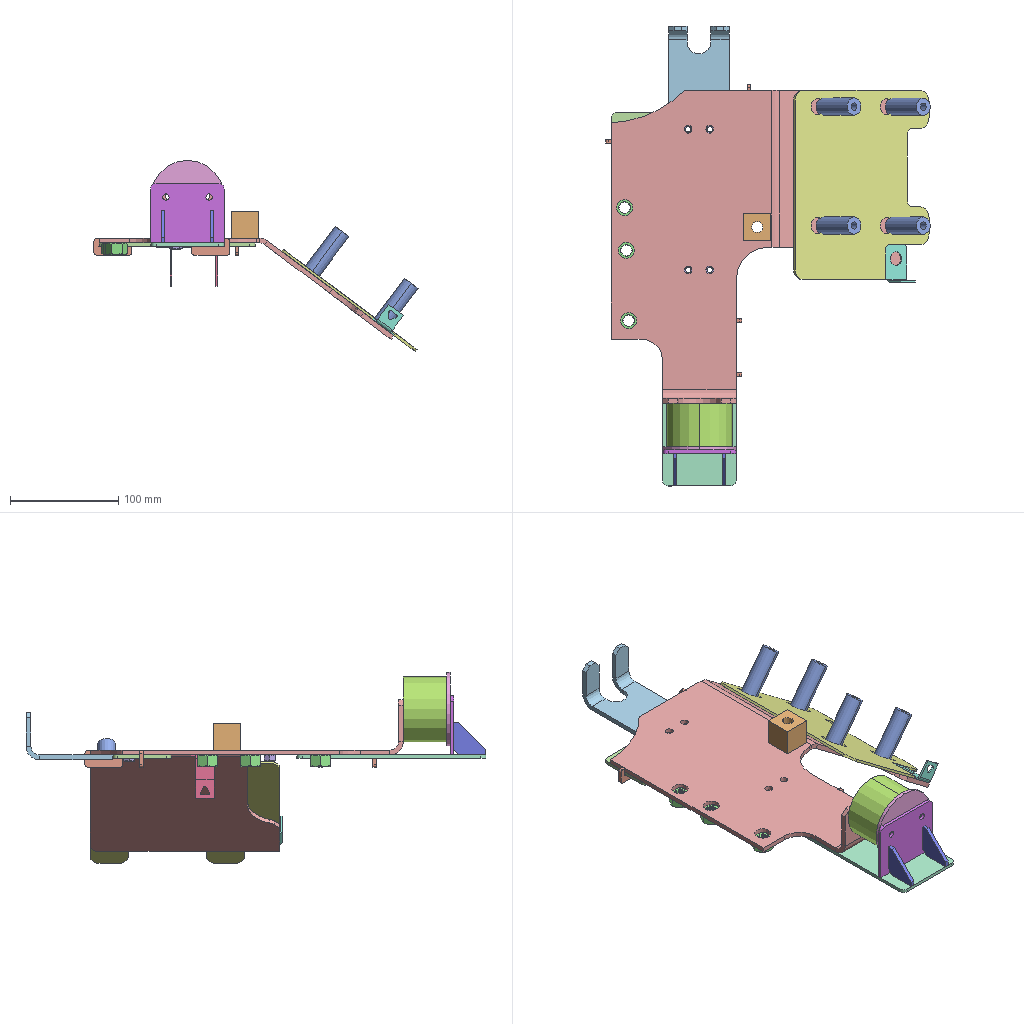Assembly | SolidWorks | 16 different items | 28 placed | box 300 x 425 x 177 mm
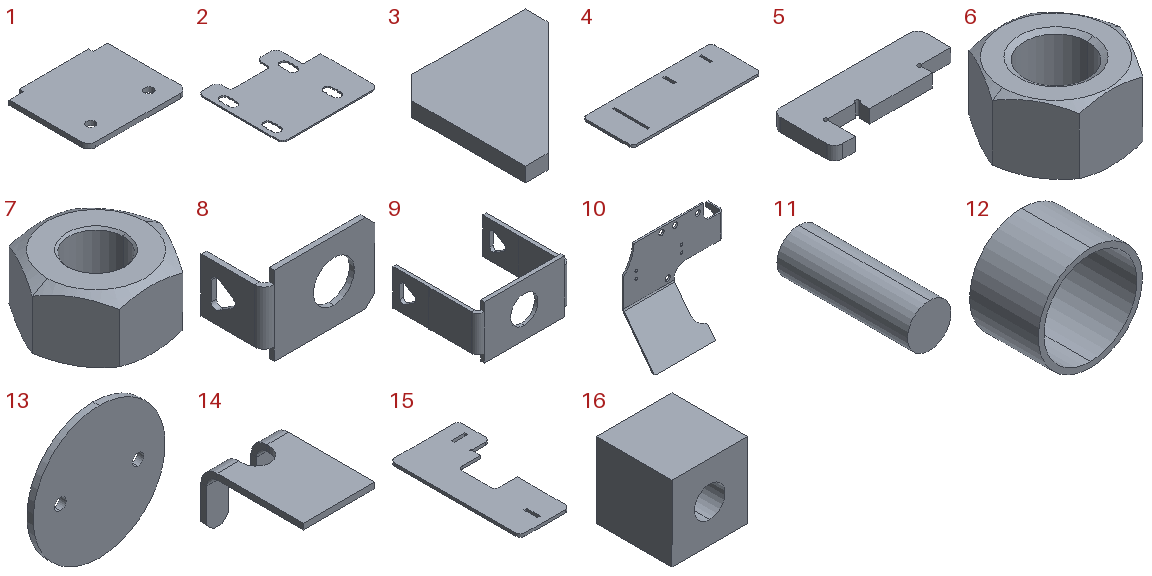Parts list (item | quantity | size | volume | features):
1 | x1 | 68 x 57.9 x 3.2 mm | 12192 mm3 | features FlatPattern 1, SMBaseFlange 1, SheetMetal 1
2 | x1 | 175 x 155 x 2.3 mm | 50413 mm3 | features FlatPattern 1, SMBaseFlange 1, SheetMetal 1
3 | x2 | 30 x 30 x 3.2 mm | 1840 mm3 | features FlatPattern 1, SMBaseFlange 1, SheetMetal 1
4 | x1 | 175 x 68 x 3.2 mm | 37213 mm3 | features FlatPattern 1, SMBaseFlange 1, SheetMetal 1
5 | x4 | 35 x 15 x 3.2 mm | 1138 mm3 | features Fillet 1, FlatPattern 1, SMBaseFlange 1, SheetMetal 1
6 | x3 | 27.713 x 24 x 14.8 mm | 5071 mm3 | features RevCut 2, Chamfer 1, Extrusion 1, LPattern 1
7 | x4 | 11.547 x 10 x 5.7 mm | 373.519 mm3 | features RevCut 4, Chamfer 2, Boss 1, Extrusion 1, LPattern 1
8 | x1 | 35 x 20 x 25 mm | 1534 mm3 | features ICE 2, Chamfer 1, FlatPattern 1, SMBaseFlange 1, SheetMetal 1
9 | x1 | 44 x 40 x 25 mm | 3354 mm3 | features ICE 6, FlatPattern 1, MirrorPattern 1, SMBaseFlange 1, SheetMetal 1
10 | x1 | 289.5 x 140.1 x 272.5 mm | 264608 mm3 | features ICE 3, Chamfer 1, EdgeFlange 1, FlatPattern 1, SMBaseFlange 1, SheetMetal 1
11 | x4 | 16 x 48 x 16 mm | 8682 mm3 | features Extrusion 1, HoleWzd 1
12 | x1 | 60.5 x 40 x 60.5 mm | 23042 mm3 | features Extrusion 1
13 | x1 | 68 x 3.2 x 68 mm | 11440 mm3 | features FlatPattern 1, SMBaseFlange 1, SheetMetal 1
14 | x1 | 56 x 80 x 44 mm | 22975 mm3 | features Chamfer 1, FlatPattern 1, ICE 1, SMBaseFlange 1, SheetMetal 1
15 | x1 | 75 x 144 x 3.2 mm | 23763 mm3 | features FlatPattern 1, SMBaseFlange 1, SheetMetal 1
16 | x1 | 25 x 25 x 25 mm | 13582 mm3 | features Extrusion 1, HoleWzd 1
Mates (type | each side: item.copy, entity, surface, feature):
Coincident | 10.1 face plane Base-Flange1 | 11.1 face plane Boss-Extrude1
DistanceDim | 11.1 face cylinder Boss-Extrude1 | 10.1 face plane Base-Flange1 | 2 times
Coincident | 10.1 face plane Edge-Flange1 | 12.1 face plane Boss-Extrude1
Concentric | 10.1 face cylinder Cut-Extrude3 | 12.1 face cylinder Boss-Extrude1
Coincident | 12.1 face plane Boss-Extrude1 | 13.1 face plane Base-Flange1
Concentric | 12.1 face cylinder Boss-Extrude1 | 13.1 face cylinder Base-Flange1
Coincident | 10.1 face plane Base-Flange1 | 8.1 face plane Base-Flange1 | 2 times
DistanceDim | 10.1 face plane Cut-Extrude2 | 8.1 face plane Cut-Extrude2
Coincident | 10.1 face plane Base-Flange1 | 16.1 face plane Boss-Extrude1
Concentric | 10.1 face cylinder Cut-Extrude1 | 16.1 face cylinder M12 Tapped Hole1
Parallel | 10.1 face plane Base-Flange1 | 16.1 face plane Boss-Extrude1
Concentric | 10.1 face cylinder Cut-Extrude1 | 7.1 face cone EndChamfer1
Coincident | 10.1 face plane Base-Flange1 | 7.1 face plane BaseNut
Concentric | 10.1 face cylinder Cut-Extrude1 | 7.2 face cone EndChamfer1
Coincident | 10.1 face plane Base-Flange1 | 7.2 face plane BaseNut
Concentric | 10.1 face cylinder Cut-Extrude1 | 7.3 face cone EndChamfer1
Coincident | 10.1 face plane Base-Flange1 | 7.3 face plane BaseNut
Concentric | 10.1 face cylinder Cut-Extrude1 | 7.4 face cone EndChamfer1
Coincident | 10.1 face plane Base-Flange1 | 7.4 face plane BaseNut
Concentric | 10.1 face cylinder Cut-Extrude1 | 6.1 face cone EndChamfer
Coincident | 10.1 face plane Base-Flange1 | 6.1 face plane BaseNut
Concentric | 10.1 face cylinder Cut-Extrude1 | 6.2 face cone EndChamfer
Coincident | 10.1 face plane Base-Flange1 | 6.2 face plane BaseNut
Concentric | 10.1 face cylinder Cut-Extrude1 | 6.3 face cone EndChamfer
Coincident | 10.1 face plane Base-Flange1 | 6.3 face plane BaseNut
Coincident | 10.1 face plane Base-Flange1 | 9.1 face plane Base-Flange1
DistanceDim | 9.1 face plane Base-Flange1 | 10.1 face plane Base-Flange1
DistanceDim | 10.1 face plane Base-Flange1 | 9.1 face plane Base-Flange1
Coincident | 10.1 face plane Base-Flange1 | 14.1 face plane Base-Flange1
DistanceDim | 14.1 face plane Base-Flange1 | 10.1 face plane Base-Flange1 | 2 times
InPlace | 10.1 face plane Base-Flange1 | 2.1 plane
Parallel | 10.1 face plane Cut-Extrude1 | 6.1 face plane BaseNut
Parallel | 10.1 face plane Cut-Extrude1 | 6.2 face plane BaseNut
Parallel | 10.1 face plane Cut-Extrude1 | 6.3 face plane BaseNut
Parallel | 10.1 face plane Cut-Extrude1 | 7.2 face plane BaseNut
Coincident | 7.1 face plane BaseNut | 7.2 face plane BaseNut
Parallel | 7.2 face plane BaseNut | 7.4 face plane BaseNut
Coincident | 7.3 face plane BaseNut | 7.4 face plane BaseNut
InPlace | 13.1 face plane Base-Flange1 | 1.1 plane
InPlace | 10.1 face plane Base-Flange1 | 4.1 plane
InPlace | 5.1 plane | assembly plane
InPlace | 3.1 plane | assembly plane
InPlace | 10.1 face plane Base-Flange1 | 15.1 plane
Coincident | 15.1 face plane Base-Flange1 | 5.2 face plane Base-Flange1 | 2 times
DistanceDim | 5.2 face plane Base-Flange1 | 15.1 face plane Base-Flange1
Coincident | 15.1 face plane Base-Flange1 | 5.3 face plane Base-Flange1 | 2 times
DistanceDim | 15.1 face plane Base-Flange1 | 5.3 face plane Base-Flange1